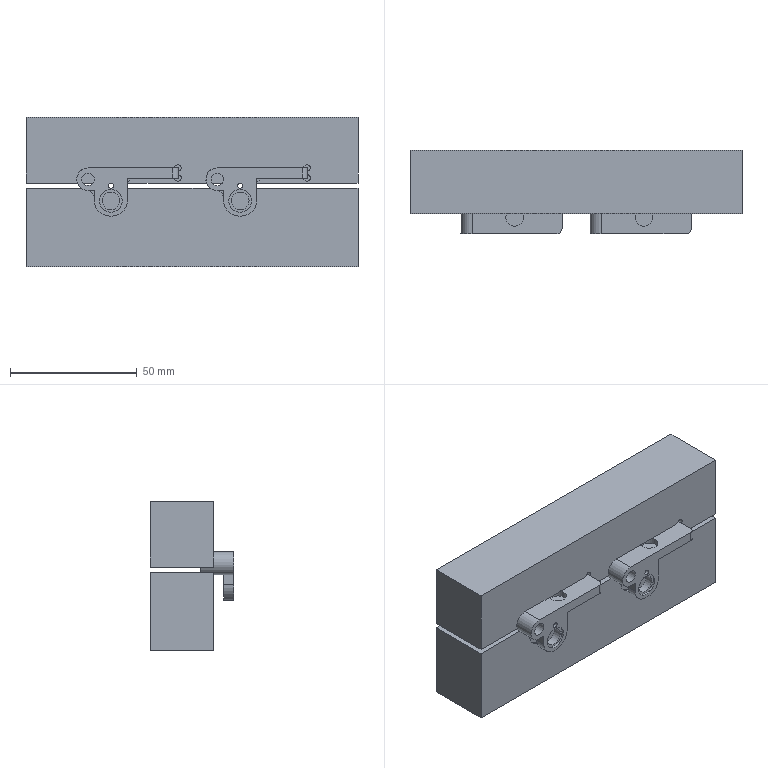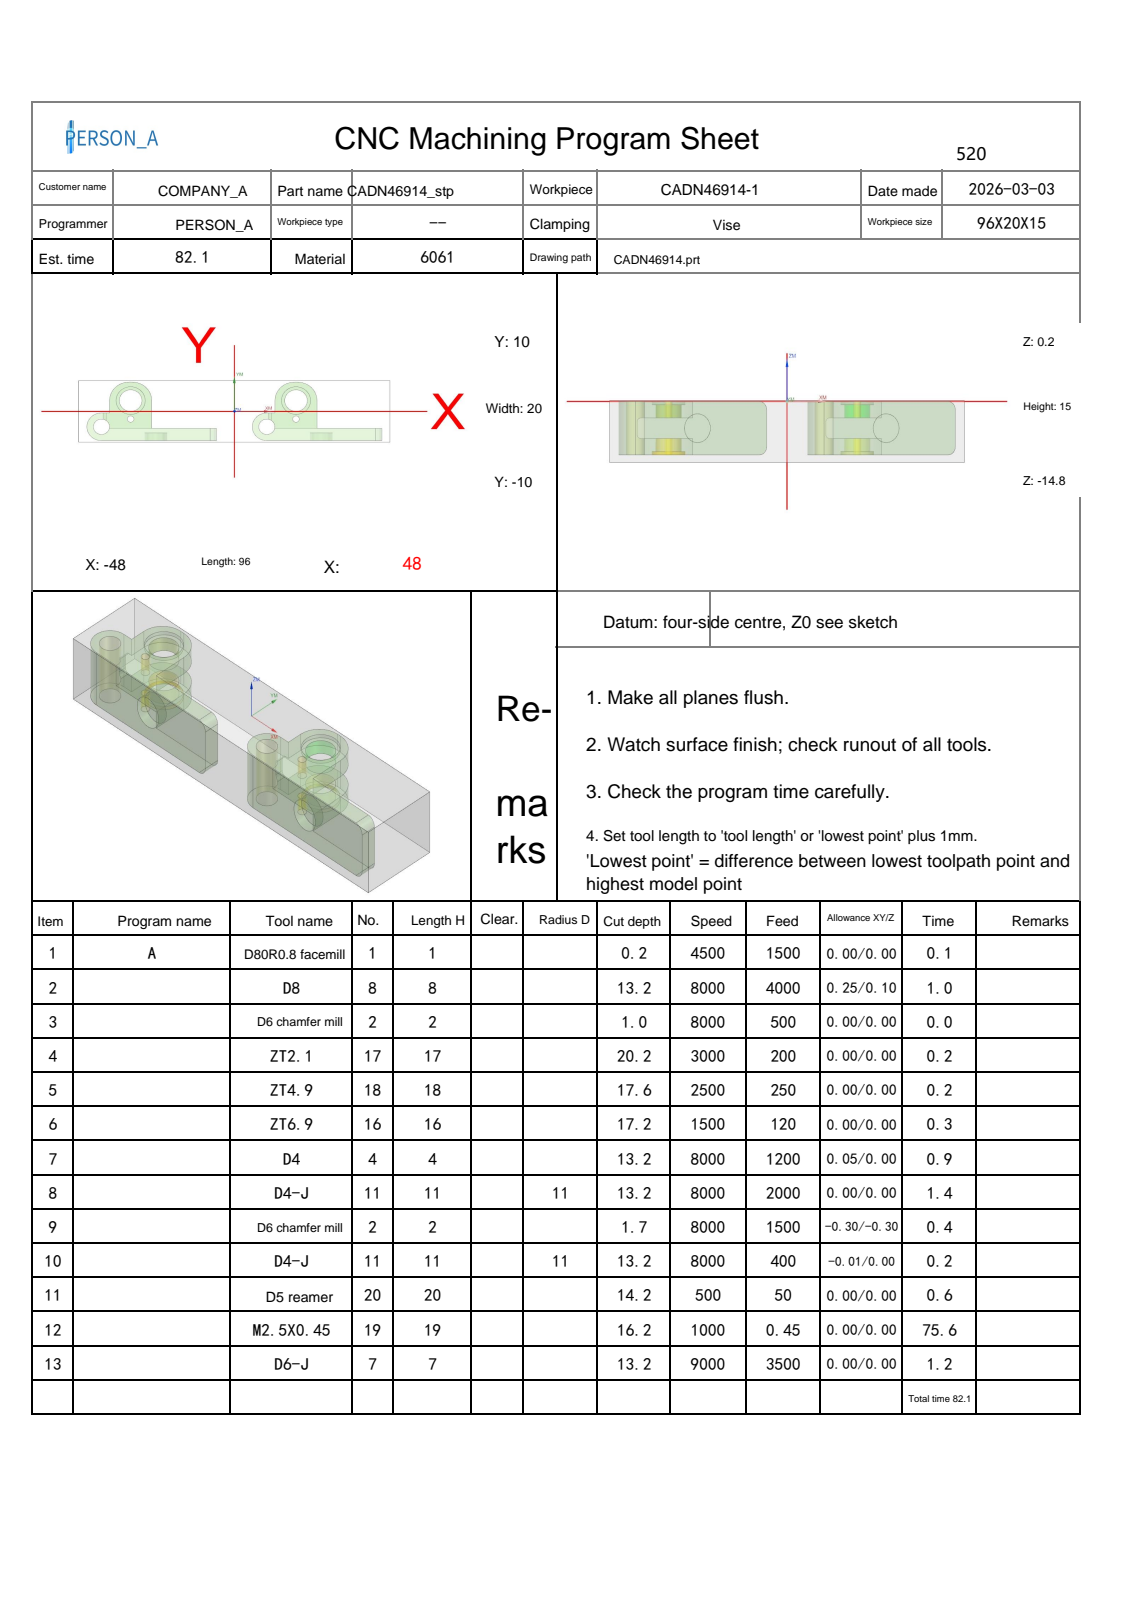NC program | NX | posted by the shop | part box 131 x 33 x 59 mm
Lines 1881 to 3020 of 12027:
N8 T11 M06
(D4-J  D=4. R=0. H=11 ce=0.00 di=0.00)
G00 G90 G54 X-32. Y3.5 M03 S8000
G43 H11 Z50.
M08
Z.5
G41 D11
G01 X-31.968 Y3.303 F500.
G03 X-30.742 Y2.258 I1.226 J.197
X-29.5 Y3.5 I0.0 J1.242
X-32.157 Y5.995 Z-.8 I-2.5 J0.0
X-34.5 Y3.5 I.157 J-2.495
X-32. Y1. I2.5 J0.0
X-29.5 Y3.5 I0.0 J2.5
X-32. Y6. I-2.5 J0.0
G01 X-32.157 Y5.995
G03 X-33.321 Y4.756 I.078 J-1.24
X-32.199 Y3.519 I1.242 J0.0
G01 G40 X-32. Y3.5
G00 Z50.
X19.
Z.5
G41 D11
G01 X19.032 Y3.303
G03 X20.258 Y2.258 I1.226 J.197
X21.5 Y3.5 I0.0 J1.242
X18.843 Y5.995 Z-.8 I-2.5 J0.0
X16.5 Y3.5 I.157 J-2.495
X19. Y1. I2.5 J0.0
X21.5 Y3.5 I0.0 J2.5
X19. Y6. I-2.5 J0.0
G01 X18.843 Y5.995
G03 X17.679 Y4.756 I.078 J-1.24
X18.801 Y3.519 I1.242 J0.0
G01 G40 X19. Y3.5
G00 Z50.
G00 G90 X7.749 Y1.536 M03 S8000
Z50.
Z.2
G01 X7.752 Y1.531 Z.139 F2000.
X7.759 Y1.518 Z.084
X7.771 Y1.498 Z.036
X7.788 Y1.473 Z-.008
X7.809 Y1.444 Z-.046
X7.834 Y1.413 Z-.079
X7.864 Y1.38 Z-.107
X7.898 Y1.348 Z-.131
X7.936 Y1.318 Z-.151
X7.978 Y1.291 Z-.167
X8.024 Y1.269 Z-.18
X8.073 Y1.254 Z-.189
X8.126 Y1.245 Z-.195
X8.183 Y1.246 Z-.199
X8.243 Y1.258 Z-.2
G02 X10. Y1.5 I1.757 J-6.258
G01 X10.5
Y3.492
X10.486 Y3.54 Z-.201
X10.445 Y3.567 Z-.203
X10.381 Y3.573 Z-.206
X10.298 Y3.561 Z-.211
X10.198 Y3.533 Z-.216
X10.084 Y3.489 Z-.223
X9.961 Y3.433 Z-.23
X9.831 Y3.365 Z-.237
X9.697 Y3.288 Z-.246
X9.563 Y3.204 Z-.254
X9.242 Y2.966 Z-.277
X8.947 Y2.697 Z-.3
X8.684 Y2.403 Z-.323
X8.461 Y2.091 Z-.346
X8.385 Y1.962 Z-.354
X8.317 Y1.835 Z-.363
X8.26 Y1.713 Z-.37
X8.213 Y1.598 Z-.378
X8.179 Y1.494 Z-.384
X8.159 Y1.405 Z-.389
X8.154 Y1.333 Z-.394
X8.166 Y1.283 Z-.397
X8.195 Y1.257 Z-.399
X8.243 Y1.258 Z-.4
G02 X10. Y1.5 I1.757 J-6.258
G01 X10.5
Y3.492
X10.486 Y3.54 Z-.401
X10.445 Y3.567 Z-.403
X10.381 Y3.573 Z-.406
X10.298 Y3.561 Z-.411
X10.198 Y3.533 Z-.416
X10.084 Y3.489 Z-.423
X9.961 Y3.433 Z-.43
X9.831 Y3.365 Z-.437
X9.697 Y3.288 Z-.446
X9.563 Y3.204 Z-.454
X9.242 Y2.966 Z-.477
X8.947 Y2.697 Z-.5
X8.684 Y2.403 Z-.523
X8.461 Y2.091 Z-.546
X8.385 Y1.962 Z-.554
X8.317 Y1.835 Z-.563
X8.26 Y1.713 Z-.57
X8.213 Y1.598 Z-.578
X8.179 Y1.494 Z-.584
X8.159 Y1.405 Z-.589
X8.154 Y1.333 Z-.594
X8.166 Y1.283 Z-.597
X8.195 Y1.257 Z-.599
X8.243 Y1.258 Z-.6
G02 X10. Y1.5 I1.757 J-6.258
G01 X10.5
Y3.492
X10.486 Y3.54 Z-.601
X10.445 Y3.567 Z-.603
X10.381 Y3.573 Z-.606
X10.298 Y3.561 Z-.611
X10.198 Y3.533 Z-.616
X10.084 Y3.489 Z-.623
X9.961 Y3.433 Z-.63
X9.831 Y3.365 Z-.637
X9.697 Y3.288 Z-.646
X9.563 Y3.204 Z-.654
X9.242 Y2.966 Z-.677
X8.947 Y2.697 Z-.7
X8.684 Y2.403 Z-.723
X8.461 Y2.091 Z-.746
X8.385 Y1.962 Z-.754
X8.317 Y1.835 Z-.763
X8.26 Y1.713 Z-.77
X8.213 Y1.598 Z-.778
X8.179 Y1.494 Z-.784
X8.159 Y1.405 Z-.789
X8.154 Y1.333 Z-.794
X8.166 Y1.283 Z-.797
X8.195 Y1.257 Z-.799
X8.243 Y1.258 Z-.8
G02 X10. Y1.5 I1.757 J-6.258
G01 X10.5
Y3.492
X10.486 Y3.54 Z-.801
X10.445 Y3.567 Z-.803
X10.381 Y3.573 Z-.806
X10.298 Y3.561 Z-.811
X10.198 Y3.533 Z-.816
X10.084 Y3.489 Z-.823
X9.961 Y3.433 Z-.83
X9.831 Y3.365 Z-.837
X9.697 Y3.288 Z-.846
X9.563 Y3.204 Z-.854
X9.242 Y2.966 Z-.877
X8.947 Y2.697 Z-.9
X8.684 Y2.403 Z-.923
X8.461 Y2.091 Z-.946
X8.385 Y1.962 Z-.954
X8.317 Y1.835 Z-.963
X8.26 Y1.713 Z-.97
X8.213 Y1.598 Z-.978
X8.179 Y1.494 Z-.984
X8.159 Y1.405 Z-.989
X8.154 Y1.333 Z-.994
X8.166 Y1.283 Z-.997
X8.195 Y1.257 Z-.999
X8.243 Y1.258 Z-1.
G02 X10. Y1.5 I1.757 J-6.258
G01 X10.5
Y3.492
X10.486 Y3.54 Z-1.001
X10.445 Y3.567 Z-1.003
X10.381 Y3.573 Z-1.006
X10.298 Y3.561 Z-1.011
X10.198 Y3.533 Z-1.016
X10.084 Y3.489 Z-1.023
X9.961 Y3.433 Z-1.03
X9.831 Y3.365 Z-1.037
X9.697 Y3.288 Z-1.046
X9.563 Y3.204 Z-1.054
X9.242 Y2.966 Z-1.077
X8.947 Y2.697 Z-1.1
X8.684 Y2.403 Z-1.123
X8.461 Y2.091 Z-1.146
X8.385 Y1.962 Z-1.154
X8.317 Y1.835 Z-1.163
X8.26 Y1.713 Z-1.17
X8.213 Y1.598 Z-1.178
X8.179 Y1.494 Z-1.184
X8.159 Y1.405 Z-1.189
X8.154 Y1.333 Z-1.194
X8.166 Y1.283 Z-1.197
X8.195 Y1.257 Z-1.199
X8.243 Y1.258 Z-1.2
G02 X10. Y1.5 I1.757 J-6.258
G01 X10.5
Y3.492
X10.486 Y3.54 Z-1.201
X10.445 Y3.567 Z-1.203
X10.381 Y3.573 Z-1.206
X10.298 Y3.561 Z-1.211
X10.198 Y3.533 Z-1.216
X10.084 Y3.489 Z-1.223
X9.961 Y3.433 Z-1.23
X9.831 Y3.365 Z-1.237
X9.697 Y3.288 Z-1.246
X9.563 Y3.204 Z-1.254
X9.242 Y2.966 Z-1.277
X8.947 Y2.697 Z-1.3
X8.684 Y2.403 Z-1.323
X8.461 Y2.091 Z-1.346
X8.385 Y1.962 Z-1.354
X8.317 Y1.835 Z-1.363
X8.26 Y1.713 Z-1.37
X8.213 Y1.598 Z-1.378
X8.179 Y1.494 Z-1.384
X8.159 Y1.405 Z-1.389
X8.154 Y1.333 Z-1.394
X8.166 Y1.283 Z-1.397
X8.195 Y1.257 Z-1.399
X8.243 Y1.258 Z-1.4
G02 X10. Y1.5 I1.757 J-6.258
G01 X10.5
Y3.492
X10.486 Y3.54 Z-1.401
X10.445 Y3.567 Z-1.403
X10.381 Y3.573 Z-1.406
X10.298 Y3.561 Z-1.411
X10.198 Y3.533 Z-1.416
X10.084 Y3.489 Z-1.423
X9.961 Y3.433 Z-1.43
X9.831 Y3.365 Z-1.437
X9.697 Y3.288 Z-1.446
X9.563 Y3.204 Z-1.454
X9.242 Y2.966 Z-1.477
X8.947 Y2.697 Z-1.5
X8.684 Y2.403 Z-1.523
X8.461 Y2.091 Z-1.546
X8.385 Y1.962 Z-1.554
X8.317 Y1.835 Z-1.563
X8.26 Y1.713 Z-1.57
X8.213 Y1.598 Z-1.578
X8.179 Y1.494 Z-1.584
X8.159 Y1.405 Z-1.589
X8.154 Y1.333 Z-1.594
X8.166 Y1.283 Z-1.597
X8.195 Y1.257 Z-1.599
X8.243 Y1.258 Z-1.6
G02 X10. Y1.5 I1.757 J-6.258
G01 X10.5
Y3.492
X10.486 Y3.54 Z-1.601
X10.445 Y3.567 Z-1.603
X10.381 Y3.573 Z-1.606
X10.298 Y3.561 Z-1.611
X10.198 Y3.533 Z-1.616
X10.084 Y3.489 Z-1.623
X9.961 Y3.433 Z-1.63
X9.831 Y3.365 Z-1.637
X9.697 Y3.288 Z-1.646
X9.563 Y3.204 Z-1.654
X9.242 Y2.966 Z-1.677
X8.947 Y2.697 Z-1.7
X8.684 Y2.403 Z-1.723
X8.461 Y2.091 Z-1.746
X8.385 Y1.962 Z-1.754
X8.317 Y1.835 Z-1.763
X8.26 Y1.713 Z-1.77
X8.213 Y1.598 Z-1.778
X8.179 Y1.494 Z-1.784
X8.159 Y1.405 Z-1.789
X8.154 Y1.333 Z-1.794
X8.166 Y1.283 Z-1.797
X8.195 Y1.257 Z-1.799
X8.243 Y1.258 Z-1.8
G02 X10. Y1.5 I1.757 J-6.258
G01 X10.5
Y3.492
X10.486 Y3.54 Z-1.801
X10.445 Y3.567 Z-1.803
X10.381 Y3.573 Z-1.806
X10.298 Y3.561 Z-1.811
X10.198 Y3.533 Z-1.816
X10.084 Y3.489 Z-1.823
X9.961 Y3.433 Z-1.83
X9.831 Y3.365 Z-1.837
X9.697 Y3.288 Z-1.846
X9.563 Y3.204 Z-1.854
X9.242 Y2.966 Z-1.877
X8.947 Y2.697 Z-1.9
X8.684 Y2.403 Z-1.923
X8.461 Y2.091 Z-1.946
X8.385 Y1.962 Z-1.954
X8.317 Y1.835 Z-1.963
X8.26 Y1.713 Z-1.97
X8.213 Y1.598 Z-1.978
X8.179 Y1.494 Z-1.984
X8.159 Y1.405 Z-1.989
X8.154 Y1.333 Z-1.994
X8.166 Y1.283 Z-1.997
X8.195 Y1.257 Z-1.999
X8.243 Y1.258 Z-2.
G02 X10. Y1.5 I1.757 J-6.258
G01 X10.5
Y3.492
X10.486 Y3.54 Z-2.001
X10.445 Y3.567 Z-2.003
X10.381 Y3.573 Z-2.006
X10.298 Y3.561 Z-2.011
X10.198 Y3.533 Z-2.016
X10.084 Y3.489 Z-2.023
X9.961 Y3.433 Z-2.03
X9.831 Y3.365 Z-2.037
X9.697 Y3.288 Z-2.046
X9.563 Y3.204 Z-2.054
X9.242 Y2.966 Z-2.077
X8.947 Y2.697 Z-2.1
X8.684 Y2.403 Z-2.123
X8.461 Y2.091 Z-2.146
X8.385 Y1.962 Z-2.154
X8.317 Y1.835 Z-2.163
X8.26 Y1.713 Z-2.17
X8.213 Y1.598 Z-2.178
X8.179 Y1.494 Z-2.184
X8.159 Y1.405 Z-2.189
X8.154 Y1.333 Z-2.194
X8.166 Y1.283 Z-2.197
X8.195 Y1.257 Z-2.199
X8.243 Y1.258 Z-2.2
G02 X10. Y1.5 I1.757 J-6.258
G01 X10.5
Y3.492
X10.486 Y3.54 Z-2.201
X10.445 Y3.567 Z-2.203
X10.381 Y3.573 Z-2.206
X10.298 Y3.561 Z-2.211
X10.198 Y3.533 Z-2.216
X10.084 Y3.489 Z-2.223
X9.961 Y3.433 Z-2.23
X9.831 Y3.365 Z-2.237
X9.697 Y3.288 Z-2.246
X9.563 Y3.204 Z-2.254
X9.242 Y2.966 Z-2.277
X8.947 Y2.697 Z-2.3
X8.684 Y2.403 Z-2.323
X8.461 Y2.091 Z-2.346
X8.385 Y1.962 Z-2.354
X8.317 Y1.835 Z-2.363
X8.26 Y1.713 Z-2.37
X8.213 Y1.598 Z-2.378
X8.179 Y1.494 Z-2.384
X8.159 Y1.405 Z-2.389
X8.154 Y1.333 Z-2.394
X8.166 Y1.283 Z-2.397
X8.195 Y1.257 Z-2.399
X8.243 Y1.258 Z-2.4
G02 X10. Y1.5 I1.757 J-6.258
G01 X10.5
Y3.492
X10.486 Y3.54 Z-2.401
X10.445 Y3.567 Z-2.403
X10.381 Y3.573 Z-2.406
X10.298 Y3.561 Z-2.411
X10.198 Y3.533 Z-2.416
X10.084 Y3.489 Z-2.423
X9.961 Y3.433 Z-2.43
X9.831 Y3.365 Z-2.437
X9.697 Y3.288 Z-2.446
X9.563 Y3.204 Z-2.454
X9.242 Y2.966 Z-2.477
X8.947 Y2.697 Z-2.5
X8.684 Y2.403 Z-2.523
X8.461 Y2.091 Z-2.546
X8.385 Y1.962 Z-2.554
X8.317 Y1.835 Z-2.563
X8.26 Y1.713 Z-2.57
X8.213 Y1.598 Z-2.578
X8.179 Y1.494 Z-2.584
X8.159 Y1.405 Z-2.589
X8.154 Y1.333 Z-2.594
X8.166 Y1.283 Z-2.597
X8.195 Y1.257 Z-2.599
X8.243 Y1.258 Z-2.6
G02 X10. Y1.5 I1.757 J-6.258
G01 X10.5
Y3.492
X10.486 Y3.54 Z-2.601
X10.445 Y3.567 Z-2.603
X10.381 Y3.573 Z-2.606
X10.298 Y3.561 Z-2.611
X10.198 Y3.533 Z-2.616
X10.084 Y3.489 Z-2.623
X9.961 Y3.433 Z-2.63
X9.831 Y3.365 Z-2.637
X9.697 Y3.288 Z-2.646
X9.563 Y3.204 Z-2.654
X9.242 Y2.966 Z-2.677
X8.947 Y2.697 Z-2.7
X8.684 Y2.403 Z-2.723
X8.461 Y2.091 Z-2.746
X8.385 Y1.962 Z-2.754
X8.317 Y1.835 Z-2.763
X8.26 Y1.713 Z-2.77
X8.213 Y1.598 Z-2.778
X8.179 Y1.494 Z-2.784
X8.159 Y1.405 Z-2.789
X8.154 Y1.333 Z-2.794
X8.166 Y1.283 Z-2.797
X8.195 Y1.257 Z-2.799
X8.243 Y1.258 Z-2.8
G02 X10. Y1.5 I1.757 J-6.258
G01 X10.5
Y3.492
X10.486 Y3.54 Z-2.801
X10.445 Y3.567 Z-2.803
X10.381 Y3.573 Z-2.806
X10.298 Y3.561 Z-2.811
X10.198 Y3.533 Z-2.816
X10.084 Y3.489 Z-2.823
X9.961 Y3.433 Z-2.83
X9.831 Y3.365 Z-2.837
X9.697 Y3.288 Z-2.846
X9.563 Y3.204 Z-2.854
X9.242 Y2.966 Z-2.877
X8.947 Y2.697 Z-2.9
X8.684 Y2.403 Z-2.923
X8.461 Y2.091 Z-2.946
X8.385 Y1.962 Z-2.954
X8.317 Y1.835 Z-2.963
X8.26 Y1.713 Z-2.97
X8.213 Y1.598 Z-2.978
X8.179 Y1.494 Z-2.984
X8.159 Y1.405 Z-2.989
X8.154 Y1.333 Z-2.994
X8.166 Y1.283 Z-2.997
X8.195 Y1.257 Z-2.999
X8.243 Y1.258 Z-3.
G02 X10. Y1.5 I1.757 J-6.258
G01 X10.5
Y3.492
X10.486 Y3.54 Z-3.001
X10.445 Y3.567 Z-3.003
X10.381 Y3.573 Z-3.006
X10.298 Y3.561 Z-3.011
X10.198 Y3.533 Z-3.016
X10.084 Y3.489 Z-3.023
X9.961 Y3.433 Z-3.03
X9.831 Y3.365 Z-3.037
X9.697 Y3.288 Z-3.046
X9.563 Y3.204 Z-3.054
X9.242 Y2.966 Z-3.077
X8.947 Y2.697 Z-3.1
X8.684 Y2.403 Z-3.123
X8.461 Y2.091 Z-3.146
X8.385 Y1.962 Z-3.154
X8.317 Y1.835 Z-3.163
X8.26 Y1.713 Z-3.17
X8.213 Y1.598 Z-3.178
X8.179 Y1.494 Z-3.184
X8.159 Y1.405 Z-3.189
X8.154 Y1.333 Z-3.194
X8.166 Y1.283 Z-3.197
X8.195 Y1.257 Z-3.199
X8.243 Y1.258 Z-3.2
G02 X10. Y1.5 I1.757 J-6.258
G01 X10.5
Y3.492
X10.486 Y3.54 Z-3.201
X10.445 Y3.567 Z-3.203
X10.381 Y3.573 Z-3.206
X10.298 Y3.561 Z-3.211
X10.198 Y3.533 Z-3.216
X10.084 Y3.489 Z-3.223
X9.961 Y3.433 Z-3.23
X9.831 Y3.365 Z-3.237
X9.697 Y3.288 Z-3.246
X9.563 Y3.204 Z-3.254
X9.242 Y2.966 Z-3.277
X8.947 Y2.697 Z-3.3
X8.684 Y2.403 Z-3.323
X8.461 Y2.091 Z-3.346
X8.385 Y1.962 Z-3.354
X8.317 Y1.835 Z-3.363
X8.26 Y1.713 Z-3.37
X8.213 Y1.598 Z-3.378
X8.179 Y1.494 Z-3.384
X8.159 Y1.405 Z-3.389
X8.154 Y1.333 Z-3.394
X8.166 Y1.283 Z-3.397
X8.195 Y1.257 Z-3.399
X8.243 Y1.258 Z-3.4
G02 X10. Y1.5 I1.757 J-6.258
G01 X10.5
Y3.492
X10.486 Y3.54 Z-3.401
X10.445 Y3.567 Z-3.403
X10.381 Y3.573 Z-3.406
X10.298 Y3.561 Z-3.411
X10.198 Y3.533 Z-3.416
X10.084 Y3.489 Z-3.423
X9.961 Y3.433 Z-3.43
X9.831 Y3.365 Z-3.437
X9.697 Y3.288 Z-3.446
X9.563 Y3.204 Z-3.454
X9.242 Y2.966 Z-3.477
X8.947 Y2.697 Z-3.5
X8.684 Y2.403 Z-3.523
X8.461 Y2.091 Z-3.546
X8.385 Y1.962 Z-3.554
X8.317 Y1.835 Z-3.563
X8.26 Y1.713 Z-3.57
X8.213 Y1.598 Z-3.578
X8.179 Y1.494 Z-3.584
X8.159 Y1.405 Z-3.589
X8.154 Y1.333 Z-3.594
X8.166 Y1.283 Z-3.597
X8.195 Y1.257 Z-3.599
X8.243 Y1.258 Z-3.6
G02 X10. Y1.5 I1.757 J-6.258
G01 X10.5
Y3.492
X10.486 Y3.54 Z-3.601
X10.445 Y3.567 Z-3.603
X10.381 Y3.573 Z-3.606
X10.298 Y3.561 Z-3.611
X10.198 Y3.533 Z-3.616
X10.084 Y3.489 Z-3.623
X9.961 Y3.433 Z-3.63
X9.831 Y3.365 Z-3.637
X9.697 Y3.288 Z-3.646
X9.563 Y3.204 Z-3.654
X9.242 Y2.966 Z-3.677
X8.947 Y2.697 Z-3.7
X8.684 Y2.403 Z-3.723
X8.461 Y2.091 Z-3.746
X8.385 Y1.962 Z-3.754
X8.317 Y1.835 Z-3.763
X8.26 Y1.713 Z-3.77
X8.213 Y1.598 Z-3.778
X8.179 Y1.494 Z-3.784
X8.159 Y1.405 Z-3.789
X8.154 Y1.333 Z-3.794
X8.166 Y1.283 Z-3.797
X8.195 Y1.257 Z-3.799
X8.243 Y1.258 Z-3.8
G02 X10. Y1.5 I1.757 J-6.258
G01 X10.5
Y3.492
X10.486 Y3.54 Z-3.801
X10.445 Y3.567 Z-3.803
X10.381 Y3.573 Z-3.806
X10.298 Y3.561 Z-3.811
X10.198 Y3.533 Z-3.816
X10.084 Y3.489 Z-3.823
X9.961 Y3.433 Z-3.83
X9.831 Y3.365 Z-3.837
X9.697 Y3.288 Z-3.846
X9.563 Y3.204 Z-3.854
X9.242 Y2.966 Z-3.877
X8.947 Y2.697 Z-3.9
X8.684 Y2.403 Z-3.923
X8.461 Y2.091 Z-3.946
X8.385 Y1.962 Z-3.954
X8.317 Y1.835 Z-3.963
X8.26 Y1.713 Z-3.97
X8.213 Y1.598 Z-3.978
X8.179 Y1.494 Z-3.984
X8.159 Y1.405 Z-3.989
X8.154 Y1.333 Z-3.994
X8.166 Y1.283 Z-3.997
X8.195 Y1.257 Z-3.999
X8.243 Y1.258 Z-4.
G02 X10. Y1.5 I1.757 J-6.258
G01 X10.5
Y3.492
X10.486 Y3.54 Z-4.001
X10.445 Y3.567 Z-4.003
X10.381 Y3.573 Z-4.006
X10.298 Y3.561 Z-4.011
X10.198 Y3.533 Z-4.016
X10.084 Y3.489 Z-4.023
X9.961 Y3.433 Z-4.03
X9.831 Y3.365 Z-4.037
X9.697 Y3.288 Z-4.046
X9.563 Y3.204 Z-4.054
X9.242 Y2.966 Z-4.077
X8.947 Y2.697 Z-4.1
X8.684 Y2.403 Z-4.123
X8.461 Y2.091 Z-4.146
X8.385 Y1.962 Z-4.154
X8.317 Y1.835 Z-4.163
X8.26 Y1.713 Z-4.17
X8.213 Y1.598 Z-4.178
X8.179 Y1.494 Z-4.184
X8.159 Y1.405 Z-4.189
X8.154 Y1.333 Z-4.194
X8.166 Y1.283 Z-4.197
X8.195 Y1.257 Z-4.199
X8.243 Y1.258 Z-4.2
G02 X10. Y1.5 I1.757 J-6.258
G01 X10.5
Y3.492
X10.486 Y3.54 Z-4.201
X10.445 Y3.567 Z-4.203
X10.381 Y3.573 Z-4.206
X10.298 Y3.561 Z-4.211
X10.198 Y3.533 Z-4.216
X10.084 Y3.489 Z-4.223
X9.961 Y3.433 Z-4.23
X9.831 Y3.365 Z-4.237
X9.697 Y3.288 Z-4.246
X9.563 Y3.204 Z-4.254
X9.242 Y2.966 Z-4.277
X8.947 Y2.697 Z-4.3
X8.684 Y2.403 Z-4.323
X8.461 Y2.091 Z-4.346
X8.385 Y1.962 Z-4.354
X8.317 Y1.835 Z-4.363
X8.26 Y1.713 Z-4.37
X8.213 Y1.598 Z-4.378
X8.179 Y1.494 Z-4.384
X8.159 Y1.405 Z-4.389
X8.154 Y1.333 Z-4.394
X8.166 Y1.283 Z-4.397
X8.195 Y1.257 Z-4.399
X8.243 Y1.258 Z-4.4
G02 X10. Y1.5 I1.757 J-6.258
G01 X10.5
Y3.492
X10.486 Y3.54 Z-4.401
X10.445 Y3.567 Z-4.403
X10.381 Y3.573 Z-4.406
X10.298 Y3.561 Z-4.411
X10.198 Y3.533 Z-4.416
X10.084 Y3.489 Z-4.423
X9.961 Y3.433 Z-4.43
X9.831 Y3.365 Z-4.437
X9.697 Y3.288 Z-4.446
X9.563 Y3.204 Z-4.454
X9.242 Y2.966 Z-4.477
X8.947 Y2.697 Z-4.5
X8.684 Y2.403 Z-4.523
X8.461 Y2.091 Z-4.546
X8.385 Y1.962 Z-4.554
X8.317 Y1.835 Z-4.563
X8.26 Y1.713 Z-4.57
X8.213 Y1.598 Z-4.578
X8.179 Y1.494 Z-4.584
X8.159 Y1.405 Z-4.589
X8.154 Y1.333 Z-4.594
X8.166 Y1.283 Z-4.597
X8.195 Y1.257 Z-4.599
X8.243 Y1.258 Z-4.6
G02 X10. Y1.5 I1.757 J-6.258
G01 X10.5
Y3.492
X10.486 Y3.54 Z-4.601
X10.445 Y3.567 Z-4.603
X10.381 Y3.573 Z-4.606
X10.298 Y3.561 Z-4.611
X10.198 Y3.533 Z-4.616
X10.084 Y3.489 Z-4.623
X9.961 Y3.433 Z-4.63
X9.831 Y3.365 Z-4.637
X9.697 Y3.288 Z-4.646
X9.563 Y3.204 Z-4.654
X9.242 Y2.966 Z-4.677
X8.947 Y2.697 Z-4.7
X8.684 Y2.403 Z-4.723
X8.461 Y2.091 Z-4.746
X8.385 Y1.962 Z-4.754
X8.317 Y1.835 Z-4.763
X8.26 Y1.713 Z-4.77
X8.213 Y1.598 Z-4.778
X8.179 Y1.494 Z-4.784
X8.159 Y1.405 Z-4.789
X8.154 Y1.333 Z-4.794
X8.166 Y1.283 Z-4.797
X8.195 Y1.257 Z-4.799
X8.243 Y1.258 Z-4.8
G02 X10. Y1.5 I1.757 J-6.258
G01 X10.5
Y3.492
X10.486 Y3.54 Z-4.801
X10.445 Y3.567 Z-4.803
X10.381 Y3.573 Z-4.806
X10.298 Y3.561 Z-4.811
X10.198 Y3.533 Z-4.816
X10.084 Y3.489 Z-4.823
X9.961 Y3.433 Z-4.83
X9.831 Y3.365 Z-4.837
X9.697 Y3.288 Z-4.846
X9.563 Y3.204 Z-4.854
X9.242 Y2.966 Z-4.877
X8.947 Y2.697 Z-4.9
X8.684 Y2.403 Z-4.923
X8.461 Y2.091 Z-4.946
X8.385 Y1.962 Z-4.954
X8.317 Y1.835 Z-4.963
X8.26 Y1.713 Z-4.97
X8.213 Y1.598 Z-4.978
X8.179 Y1.494 Z-4.984
X8.159 Y1.405 Z-4.989
X8.154 Y1.333 Z-4.994
X8.166 Y1.283 Z-4.997
X8.195 Y1.257 Z-4.999
X8.243 Y1.258 Z-5.
G02 X10. Y1.5 I1.757 J-6.258
G01 X10.5
Y3.492
X10.486 Y3.54 Z-5.001
X10.445 Y3.567 Z-5.003
X10.381 Y3.573 Z-5.006
X10.298 Y3.561 Z-5.011
X10.198 Y3.533 Z-5.016
X10.084 Y3.489 Z-5.023
X9.961 Y3.433 Z-5.03
X9.831 Y3.365 Z-5.037
X9.697 Y3.288 Z-5.046
X9.563 Y3.204 Z-5.054
X9.242 Y2.966 Z-5.077
X8.947 Y2.697 Z-5.1
X8.684 Y2.403 Z-5.123
X8.461 Y2.091 Z-5.146
X8.385 Y1.962 Z-5.154
X8.317 Y1.835 Z-5.163
X8.26 Y1.713 Z-5.17
X8.213 Y1.598 Z-5.178
X8.179 Y1.494 Z-5.184
X8.159 Y1.405 Z-5.189
X8.154 Y1.333 Z-5.194
X8.166 Y1.283 Z-5.197
X8.195 Y1.257 Z-5.199
X8.243 Y1.258 Z-5.2
G02 X10. Y1.5 I1.757 J-6.258
G01 X10.5
Y3.492
X10.486 Y3.54 Z-5.201
X10.445 Y3.567 Z-5.203
X10.381 Y3.573 Z-5.206
X10.298 Y3.561 Z-5.211
X10.198 Y3.533 Z-5.216
X10.084 Y3.489 Z-5.223
X9.961 Y3.433 Z-5.23
X9.831 Y3.365 Z-5.237
X9.697 Y3.288 Z-5.246
X9.563 Y3.204 Z-5.254
X9.242 Y2.966 Z-5.277
X8.947 Y2.697 Z-5.3
X8.684 Y2.403 Z-5.323
X8.461 Y2.091 Z-5.346
X8.385 Y1.962 Z-5.354
X8.317 Y1.835 Z-5.363
X8.26 Y1.713 Z-5.37
X8.213 Y1.598 Z-5.378
X8.179 Y1.494 Z-5.384
X8.159 Y1.405 Z-5.389
X8.154 Y1.333 Z-5.394
X8.166 Y1.283 Z-5.397
X8.195 Y1.257 Z-5.399
X8.243 Y1.258 Z-5.4
G02 X10. Y1.5 I1.757 J-6.258
G01 X10.5
Y3.492
X10.486 Y3.54 Z-5.401
X10.445 Y3.567 Z-5.403
X10.381 Y3.573 Z-5.406
X10.298 Y3.561 Z-5.411
X10.198 Y3.533 Z-5.416
X10.084 Y3.489 Z-5.423
X9.961 Y3.433 Z-5.43
X9.831 Y3.365 Z-5.437
X9.697 Y3.288 Z-5.446
X9.563 Y3.204 Z-5.454
X9.242 Y2.966 Z-5.477
X8.947 Y2.697 Z-5.5
X8.684 Y2.403 Z-5.523
X8.461 Y2.091 Z-5.546
X8.385 Y1.962 Z-5.554
X8.317 Y1.835 Z-5.563
X8.26 Y1.713 Z-5.57
X8.213 Y1.598 Z-5.578
X8.179 Y1.494 Z-5.584
X8.159 Y1.405 Z-5.589
X8.154 Y1.333 Z-5.594
X8.166 Y1.283 Z-5.597
X8.195 Y1.257 Z-5.599
X8.243 Y1.258 Z-5.6
G02 X10. Y1.5 I1.757 J-6.258
G01 X10.5
Y3.492
X10.486 Y3.54 Z-5.601
X10.445 Y3.567 Z-5.603
X10.381 Y3.573 Z-5.606
X10.298 Y3.561 Z-5.611
X10.198 Y3.533 Z-5.616
X10.084 Y3.489 Z-5.623
X9.961 Y3.433 Z-5.63
X9.831 Y3.365 Z-5.637
X9.697 Y3.288 Z-5.646
X9.563 Y3.204 Z-5.654
X9.242 Y2.966 Z-5.677
X8.947 Y2.697 Z-5.7
X8.684 Y2.403 Z-5.723
X8.461 Y2.091 Z-5.746
X8.385 Y1.962 Z-5.754
X8.317 Y1.835 Z-5.763
X8.26 Y1.713 Z-5.77
X8.213 Y1.598 Z-5.778
X8.179 Y1.494 Z-5.784
X8.159 Y1.405 Z-5.789
X8.154 Y1.333 Z-5.794
X8.166 Y1.283 Z-5.797
X8.195 Y1.257 Z-5.799
X8.243 Y1.258 Z-5.8
G02 X10. Y1.5 I1.757 J-6.258
G01 X10.5
Y3.492
X10.486 Y3.54 Z-5.801
X10.445 Y3.567 Z-5.803
X10.381 Y3.573 Z-5.806
X10.298 Y3.561 Z-5.811
X10.198 Y3.533 Z-5.816
X10.084 Y3.489 Z-5.823
X9.961 Y3.433 Z-5.83
X9.831 Y3.365 Z-5.837
X9.697 Y3.288 Z-5.846
X9.563 Y3.204 Z-5.854
X9.242 Y2.966 Z-5.877
X8.947 Y2.697 Z-5.9
X8.684 Y2.403 Z-5.923
X8.461 Y2.091 Z-5.946
X8.385 Y1.962 Z-5.954
X8.317 Y1.835 Z-5.963
X8.26 Y1.713 Z-5.97
X8.213 Y1.598 Z-5.978
X8.179 Y1.494 Z-5.984
X8.159 Y1.405 Z-5.989
X8.154 Y1.333 Z-5.994
X8.166 Y1.283 Z-5.997
X8.195 Y1.257 Z-5.999
X8.243 Y1.258 Z-6.
G02 X10. Y1.5 I1.757 J-6.258
G01 X10.5
Y3.492
X10.486 Y3.54 Z-6.001
X10.445 Y3.567 Z-6.003
X10.381 Y3.573 Z-6.006
X10.298 Y3.561 Z-6.011
X10.198 Y3.533 Z-6.016
X10.084 Y3.489 Z-6.023
X9.961 Y3.433 Z-6.03
X9.831 Y3.365 Z-6.037
X9.697 Y3.288 Z-6.046
X9.563 Y3.204 Z-6.054
X9.242 Y2.966 Z-6.077
X8.947 Y2.697 Z-6.1
X8.684 Y2.403 Z-6.123
X8.461 Y2.091 Z-6.146
X8.385 Y1.962 Z-6.154
X8.317 Y1.835 Z-6.163
X8.26 Y1.713 Z-6.17
X8.213 Y1.598 Z-6.178
X8.179 Y1.494 Z-6.184
X8.159 Y1.405 Z-6.189
X8.154 Y1.333 Z-6.194
X8.166 Y1.283 Z-6.197
X8.195 Y1.257 Z-6.199
X8.243 Y1.258 Z-6.2
G02 X10. Y1.5 I1.757 J-6.258
G01 X10.5
Y3.492
X10.486 Y3.54 Z-6.201
X10.445 Y3.567 Z-6.203
X10.381 Y3.573 Z-6.206
X10.298 Y3.561 Z-6.211
X10.198 Y3.533 Z-6.216
X10.084 Y3.489 Z-6.223
X9.961 Y3.433 Z-6.23
X9.831 Y3.365 Z-6.237
X9.697 Y3.288 Z-6.246
X9.563 Y3.204 Z-6.254
X9.242 Y2.966 Z-6.277
X8.947 Y2.697 Z-6.3
X8.684 Y2.403 Z-6.323
X8.461 Y2.091 Z-6.346
X8.385 Y1.962 Z-6.354
X8.317 Y1.835 Z-6.363
X8.26 Y1.713 Z-6.37
X8.213 Y1.598 Z-6.378
X8.179 Y1.494 Z-6.384
X8.159 Y1.405 Z-6.389
X8.154 Y1.333 Z-6.394
X8.166 Y1.283 Z-6.397
X8.195 Y1.257 Z-6.399
X8.243 Y1.258 Z-6.4
G02 X10. Y1.5 I1.757 J-6.258
G01 X10.5
Y3.492
X10.486 Y3.54 Z-6.401
X10.445 Y3.567 Z-6.403
X10.381 Y3.573 Z-6.406
X10.298 Y3.561 Z-6.411
X10.198 Y3.533 Z-6.416
X10.084 Y3.489 Z-6.423
X9.961 Y3.433 Z-6.43
X9.831 Y3.365 Z-6.437
X9.697 Y3.288 Z-6.446
X9.563 Y3.204 Z-6.454
X9.242 Y2.966 Z-6.477
X8.947 Y2.697 Z-6.5
X8.684 Y2.403 Z-6.523
X8.461 Y2.091 Z-6.546
X8.385 Y1.962 Z-6.554
X8.317 Y1.835 Z-6.563
X8.26 Y1.713 Z-6.57
X8.213 Y1.598 Z-6.578
X8.179 Y1.494 Z-6.584
X8.159 Y1.405 Z-6.589
X8.154 Y1.333 Z-6.594
X8.166 Y1.283 Z-6.597
X8.195 Y1.257 Z-6.599
X8.243 Y1.258 Z-6.6
G02 X10. Y1.5 I1.757 J-6.258
G01 X10.5
Y3.492
X10.486 Y3.54 Z-6.601
X10.445 Y3.567 Z-6.603
X10.381 Y3.573 Z-6.606
X10.298 Y3.561 Z-6.611
X10.198 Y3.533 Z-6.616
X10.084 Y3.489 Z-6.623
X9.961 Y3.433 Z-6.63
X9.831 Y3.365 Z-6.637
X9.697 Y3.288 Z-6.646
X9.563 Y3.204 Z-6.654
X9.242 Y2.966 Z-6.677
X8.947 Y2.697 Z-6.7
X8.684 Y2.403 Z-6.723
X8.461 Y2.091 Z-6.746
X8.385 Y1.962 Z-6.754
X8.317 Y1.835 Z-6.763
X8.26 Y1.713 Z-6.77
X8.213 Y1.598 Z-6.778
X8.179 Y1.494 Z-6.784
X8.159 Y1.405 Z-6.789
X8.154 Y1.333 Z-6.794
X8.166 Y1.283 Z-6.797
X8.195 Y1.257 Z-6.799
X8.243 Y1.258 Z-6.8
G02 X10. Y1.5 I1.757 J-6.258
G01 X10.5
Y3.492
X10.486 Y3.54 Z-6.801
X10.445 Y3.567 Z-6.803
X10.381 Y3.573 Z-6.806
X10.298 Y3.561 Z-6.811
X10.198 Y3.533 Z-6.816
X10.084 Y3.489 Z-6.823
X9.961 Y3.433 Z-6.83
X9.831 Y3.365 Z-6.837
X9.697 Y3.288 Z-6.846
X9.563 Y3.204 Z-6.854
X9.242 Y2.966 Z-6.877
X8.947 Y2.697 Z-6.9
X8.684 Y2.403 Z-6.923
X8.461 Y2.091 Z-6.946
X8.385 Y1.962 Z-6.954
X8.317 Y1.835 Z-6.963
X8.26 Y1.713 Z-6.97
X8.213 Y1.598 Z-6.978
X8.179 Y1.494 Z-6.984
X8.159 Y1.405 Z-6.989
X8.154 Y1.333 Z-6.994
X8.166 Y1.283 Z-6.997
X8.195 Y1.257 Z-6.999
X8.243 Y1.258 Z-7.
G02 X10. Y1.5 I1.757 J-6.258
G01 X10.5
Y3.492
X10.486 Y3.54 Z-7.001
X10.445 Y3.567 Z-7.003
X10.381 Y3.573 Z-7.006
X10.298 Y3.561 Z-7.011
X10.198 Y3.533 Z-7.016
X10.084 Y3.489 Z-7.023
X9.961 Y3.433 Z-7.03
X9.831 Y3.365 Z-7.037
X9.697 Y3.288 Z-7.046
X9.563 Y3.204 Z-7.054
X9.242 Y2.966 Z-7.077
X8.947 Y2.697 Z-7.1
X8.684 Y2.403 Z-7.123
X8.461 Y2.091 Z-7.146
X8.385 Y1.962 Z-7.154
X8.317 Y1.835 Z-7.163
X8.26 Y1.713 Z-7.17
X8.213 Y1.598 Z-7.178
X8.179 Y1.494 Z-7.184
X8.159 Y1.405 Z-7.189
X8.154 Y1.333 Z-7.194
X8.166 Y1.283 Z-7.197
X8.195 Y1.257 Z-7.199
X8.243 Y1.258 Z-7.2
G02 X10. Y1.5 I1.757 J-6.258
G01 X10.5
Y3.492
X10.486 Y3.54 Z-7.201
X10.445 Y3.567 Z-7.203
X10.381 Y3.573 Z-7.206
X10.298 Y3.561 Z-7.211
X10.198 Y3.533 Z-7.216
X10.084 Y3.489 Z-7.223
X9.961 Y3.433 Z-7.23
X9.831 Y3.365 Z-7.237
X9.697 Y3.288 Z-7.246
X9.563 Y3.204 Z-7.254
X9.242 Y2.966 Z-7.277
X8.947 Y2.697 Z-7.3
X8.684 Y2.403 Z-7.323
X8.461 Y2.091 Z-7.346
X8.385 Y1.962 Z-7.354
X8.317 Y1.835 Z-7.363
X8.26 Y1.713 Z-7.37
X8.213 Y1.598 Z-7.378
X8.179 Y1.494 Z-7.384
X8.159 Y1.405 Z-7.389
X8.154 Y1.333 Z-7.394
X8.166 Y1.283 Z-7.397
X8.195 Y1.257 Z-7.399
X8.243 Y1.258 Z-7.4
G02 X10. Y1.5 I1.757 J-6.258
G01 X10.5
Y3.492
X10.486 Y3.54 Z-7.401
X10.445 Y3.567 Z-7.403
X10.381 Y3.573 Z-7.406
X10.298 Y3.561 Z-7.411
X10.198 Y3.533 Z-7.416
X10.084 Y3.489 Z-7.423
X9.961 Y3.433 Z-7.43
X9.831 Y3.365 Z-7.437
X9.697 Y3.288 Z-7.446
X9.563 Y3.204 Z-7.454
X9.242 Y2.966 Z-7.477
X8.947 Y2.697 Z-7.5
X8.684 Y2.403 Z-7.523
X8.461 Y2.091 Z-7.546
X8.385 Y1.962 Z-7.554
X8.317 Y1.835 Z-7.563
X8.26 Y1.713 Z-7.57
X8.213 Y1.598 Z-7.578
X8.179 Y1.494 Z-7.584
X8.159 Y1.405 Z-7.589
X8.154 Y1.333 Z-7.594
X8.166 Y1.283 Z-7.597
X8.195 Y1.257 Z-7.599
X8.243 Y1.258 Z-7.6
G02 X10. Y1.5 I1.757 J-6.258
G01 X10.5
Y3.492
X10.486 Y3.54 Z-7.601
X10.445 Y3.567 Z-7.603
X10.381 Y3.573 Z-7.606
X10.298 Y3.561 Z-7.611
X10.198 Y3.533 Z-7.616
X10.084 Y3.489 Z-7.623
X9.961 Y3.433 Z-7.63
X9.831 Y3.365 Z-7.637
X9.697 Y3.288 Z-7.646
X9.563 Y3.204 Z-7.654
X9.242 Y2.966 Z-7.677
X8.947 Y2.697 Z-7.7
X8.684 Y2.403 Z-7.723
X8.461 Y2.091 Z-7.746
X8.385 Y1.962 Z-7.754
X8.317 Y1.835 Z-7.763
X8.26 Y1.713 Z-7.77
X8.213 Y1.598 Z-7.778
X8.179 Y1.494 Z-7.784
X8.159 Y1.405 Z-7.789
X8.154 Y1.333 Z-7.794
X8.166 Y1.283 Z-7.797
X8.195 Y1.257 Z-7.799
X8.243 Y1.258 Z-7.8
G02 X10. Y1.5 I1.757 J-6.258
G01 X10.5
Y3.492
X10.486 Y3.54 Z-7.801
X10.445 Y3.567 Z-7.803
X10.381 Y3.573 Z-7.806
X10.298 Y3.561 Z-7.811
X10.198 Y3.533 Z-7.816
X10.084 Y3.489 Z-7.823
X9.961 Y3.433 Z-7.83
X9.831 Y3.365 Z-7.837
X9.697 Y3.288 Z-7.846
X9.563 Y3.204 Z-7.854
X9.242 Y2.966 Z-7.877
X8.947 Y2.697 Z-7.9
X8.684 Y2.403 Z-7.923
X8.461 Y2.091 Z-7.946
X8.385 Y1.962 Z-7.954
X8.317 Y1.835 Z-7.963
X8.26 Y1.713 Z-7.97
X8.213 Y1.598 Z-7.978
X8.179 Y1.494 Z-7.984
X8.159 Y1.405 Z-7.989
X8.154 Y1.333 Z-7.994
X8.166 Y1.283 Z-7.997
X8.195 Y1.257 Z-7.999
X8.243 Y1.258 Z-8.
G02 X10. Y1.5 I1.757 J-6.258
G01 X10.5
Y3.492
X10.486 Y3.54 Z-8.001
X10.445 Y3.567 Z-8.003
X10.381 Y3.573 Z-8.006
X10.298 Y3.561 Z-8.011
X10.198 Y3.533 Z-8.016
X10.084 Y3.489 Z-8.023
X9.961 Y3.433 Z-8.03
X9.831 Y3.365 Z-8.037
X9.697 Y3.288 Z-8.046
X9.563 Y3.204 Z-8.054
X9.242 Y2.966 Z-8.077
X8.947 Y2.697 Z-8.1
X8.684 Y2.403 Z-8.123
X8.461 Y2.091 Z-8.146
X8.385 Y1.962 Z-8.154
X8.317 Y1.835 Z-8.163
X8.26 Y1.713 Z-8.17
X8.213 Y1.598 Z-8.178
X8.179 Y1.494 Z-8.184
X8.159 Y1.405 Z-8.189
X8.154 Y1.333 Z-8.194
X8.166 Y1.283 Z-8.197
X8.195 Y1.257 Z-8.199
X8.243 Y1.258 Z-8.2
G02 X10. Y1.5 I1.757 J-6.258
G01 X10.5
Y3.492
X10.486 Y3.54 Z-8.201
X10.445 Y3.567 Z-8.203
X10.381 Y3.573 Z-8.206